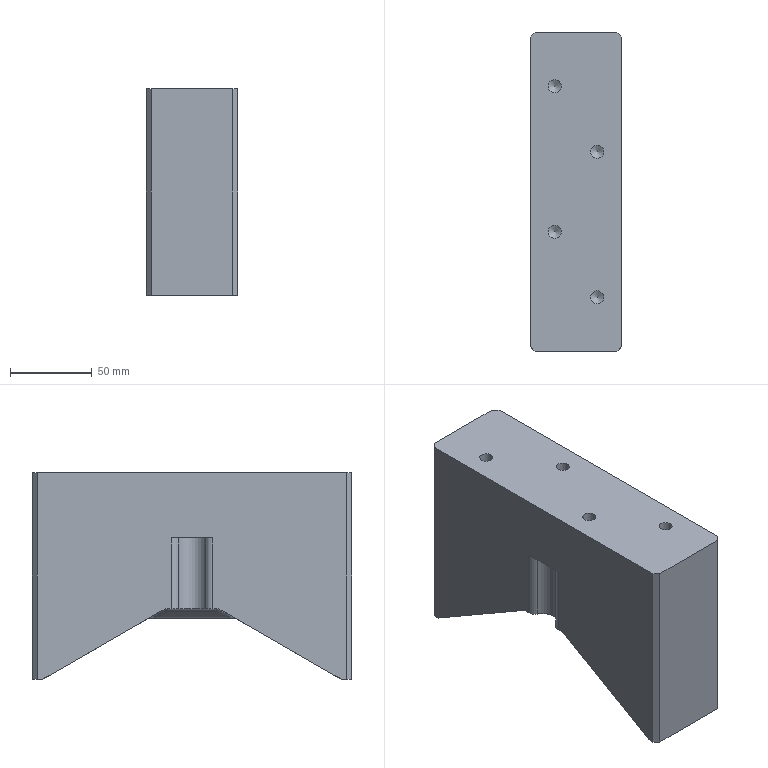Part | STEP file | 1_id74_x_t | 1 solid | 70 faces | box 56 x 195 x 126 mm | volume 1101348 mm3 | spline 24 | plane 18 | cylinder 16 | sphere 8 | cone 4 | commonest cylinder face diameters 7.938 x4 10 x4 5.85 x2 12 x2 12.3 x2 18 x2